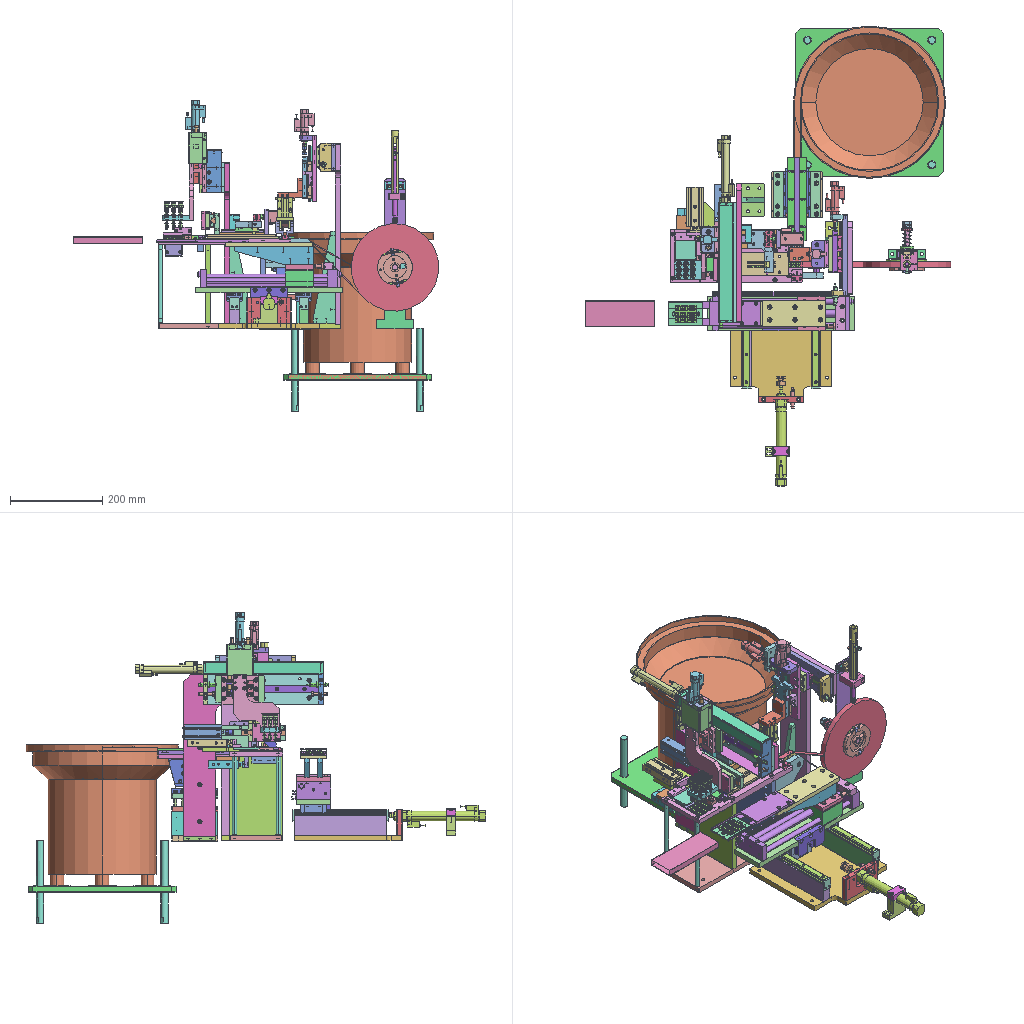Assembly | STEP file | 163 different items | 250 placed | box 792 x 996 x 674 mm
Parts list (item | name | quantity | parent item | size | volume):
1 | PN_0001 Mount electronic clip base plate | x1 | - | 115 x 233 x 12 mm | 313239 mm3
2 | PN_0002 Mount electronic clip base support plate A | x1 | - | 115 x 172 x 12 mm | 235166 mm3
3 | PN_0003 Mount electronic clip support plate B | x1 | - | 115 x 172 x 12 mm | 236361 mm3
4 | PN_0004 Mount electronic clip guide groove block | x1 | - | 287 x 115 x 14 mm | 343066 mm3
5 | PN_0005 Mount electronic clip support shaft | x2 | - | 10 x 10 x 171 mm | 13199 mm3
6 | PN_0006 Mount electronic clip pad block 3 | x1 | - | 99 x 40 x 13 mm | 46951 mm3
7 | PN_0007 Mount electronic clip cylinder mounting plate 1 | x1 | - | 40 x 62 x 8 mm | 17667 mm3
8 | PN_0008 Mount electronic clip movable head A | x1 | - | 10 x 10 x 30 mm | 1030 mm3
9 | PN_0009 Mount electronic clip movable connector head B | x1 | - | 36 x 16 x 18 mm | 5496 mm3
10 | PN_0010 Mount electronic clip quantitative slide block | x1 | - | 90 x 58 x 12 mm | 32694 mm3
11 | PN_0011 Mount electronic clip block | x1 | - | 14 x 34.832 x 10 mm | 2899 mm3
12 | PN_0012 Mount electronic clip wheel shaft A | x1 | - | 5 x 5 x 38 mm | 723.858 mm3
13 | PN_0013 Mount electronic clip mounting plate 1 | x1 | - | 160 x 54 x 10 mm | 58459 mm3
14 | PN_0014 Mount electronic clip cylinder pad block | x1 | - | 22 x 32 x 6 mm | 4030 mm3
15 | PN_0015 Mount electronic clip cylinder connecting head | x1 | - | 14 x 14 x 19 mm | 1465 mm3
16 | PN_0016 Mount electronic clip connecting block | x1 | - | 40 x 10 x 70 mm | 23648 mm3
17 | PN_0017 Mount electronic clip blade pressure plate 2 | x1 | - | 40 x 8 x 60 mm | 18433 mm3
18 | PN_0018 Mount electronic clip limit block B | x1 | - | 22 x 50 x 40 mm | 16406 mm3
19 | PN_0019 Mount electronic clip transparent acrylic cover plate | x1 | - | 152 x 50 x 8 mm | 50516 mm3
20 | PN_0021 Mount electronic clip pressure block | x2 | - | 14 x 15 x 9 mm | 1490 mm3
21 | PN_0022 Mount electronic clip pressure block | x1 | - | 22 x 8 x 31 mm | 3731 mm3
22 | PN_0023 Mount electronic clip pressure plate | x1 | - | 40 x 16 x 10 mm | 4854 mm3
23 | PN_0024 Mount electronic clip spring mounting plate | x1 | - | 54 x 12 x 15 mm | 8265 mm3
24 | PN_0025 Mount electronic clip cylinder mounting plate 4 | x1 | - | 61 x 80 x 10 mm | 39986 mm3
25 | PN_0026 Mount electronic clip cylinder connecting plate | x1 | - | 60 x 18 x 18 mm | 7277 mm3
26 | PN_0027 Mount electronic clip acrylic plate | x1 | - | 44 x 56 x 5 mm | 11600 mm3
27 | PN_0028 Mount electronic clip mounting plate 3 | x1 | - | 50 x 40 x 9 mm | 17291 mm3
28 | PN_0029 Mount electronic clip connecting plate 1 | x1 | - | 43 x 36 x 35 mm | 15801 mm3
29 | PN_0030 Mount electronic clip fiber mounting seat A | x1 | - | 22 x 18 x 8 mm | 1490 mm3
30 | PN_0031 Mount electronic clip fiber sensor seat B | x1 | - | 23 x 10 x 10 mm | 1376 mm3
31 | PN_0032 Mount electronic clip wheel connecting mounting plate | x1 | - | 98 x 64 x 12 mm | 54471 mm3
32 | PN_0033 Mount electronic clip wheel connector | x1 | - | 34 x 34 x 16.4 mm | 6483 mm3
33 | PN_0034 Mount electronic clip support wheel shaft | x1 | - | 12 x 12 x 41.3 mm | 3359 mm3
34 | PN_0038 vibratory adjusting plate A | x1 | in AAAACcBASE vibratory feeder assembly B | 100 x 100 x 10 mm | 94670 mm3
35 | PN_0037 vibratory adjusting plate B | x1 | in AAAACcBASE vibratory feeder assembly B | 100 x 10 x 100 mm | 97001 mm3
36 | A vibratory feeder 1 | x1 | in AAAA upper machine frame component | 108 x 76 x 60.4 mm | 290957 mm3
37 | ASCB6-30 | x8 | in AAAA upper machine frame component | 36 x 10 x 10 mm | 1241 mm3
38 | PN_0039 vibratory feeder connecting plate | x1 | in AAAA upper machine frame component | 140 x 8 x 40 mm | 43075 mm3
39 | PN_0036 vibratory vertical plate | x2 | in AAAA upper machine frame component | 100 x 10 x 55 mm | 54201 mm3
40 | PN_0035 vibratory base plate | x1 | in AAAA upper machine frame component | 110 x 100 x 12 mm | 122022 mm3
41 | PN_0040 linear vibrating groove | x1 | - | 180 x 40 x 10 mm | 61766 mm3
42 | PN_0041 Mount electronic clip pressure rod | x2 | - | 15 x 180 x 3 mm | 7714 mm3
43 | PN_0042 Mount electronic clip fixed groove | x1 | - | 25 x 7.5 x 40 mm | 5632 mm3
44 | PN_0043 Mount electronic clip pressure block A | x2 | - | 7.5 x 20 x 4 mm | 440.722 mm3
45 | PN_0044 Mount electronic clip mounting base plate B | x1 | - | 60 x 80 x 12 mm | 51231 mm3
46 | PN_0045 Mount electronic clip mounting plate 6 | x1 | - | 160 x 392 x 12 mm | 427849 mm3
47 | PN_0046 Mount electronic clip reinforcing rib A | x2 | - | 48 x 200 x 10 mm | 59178 mm3
48 | Mount electronic clip vibrating plate BM23-2V1 part | x1 | - | 330 x 330 x 319 mm | 10354356 mm3
49 | PN_0047 Mount electronic clip mounting base plate | x1 | in Mount electronic clip manipulator A | 60 x 10 x 175 mm | 99342 mm3
50 | MGN12C (slide rail) | x1 | in Mount electronic clip manipulator A | 12 x 8 x 145 mm | 12355 mm3
51 | Mount electronic clip MGN12C (slider) | x2 | in Mount electronic clip manipulator A | 27 x 10 x 34.7 mm | 7013 mm3
52 | PN_0048 Mount electronic clip cylinder mounting plate | x1 | in Mount electronic clip manipulator A | 60 x 28 x 10 mm | 13235 mm3
53 | PN_0049 Mount electronic clip cylinder mounting plate 2 | x1 | in Mount electronic clip manipulator A | 60 x 25 x 10 mm | 13990 mm3
54 | PN_0050 Mount electronic clip slider mounting plate | x1 | in Mount electronic clip manipulator A | 90 x 58 x 10 mm | 36578 mm3
55 | Mount electronic clip RB0806 | x2 | in Mount electronic clip manipulator A | 12 x 13.856 x 46.8 mm | 2563 mm3
56 | Mount electronic clip cylinder CDJ2B16-30-C76(0) | x1 | in Mount electronic clip manipulator A | 18.6 x 41.8 x 105 mm | 26186 mm3
57 | PN_0051 Mount electronic clip movable connector head | x2 | in Mount electronic clip manipulator A, Mount electronic clip manipulator A Z-axis | 10 x 10 x 18 mm | 883.594 mm3
58 | PN_0052 Mount electronic clip manipulator mounting plate | x1 | - | 45 x 80 x 10 mm | 30659 mm3
59 | PN_0053 Mount electronic clip mounting base plate Z-axis | x1 | in Mount electronic clip manipulator A Z-axis | 60 x 10 x 144 mm | 79878 mm3
60 | Mount electronic clip MGN12C (slide rail) Z-axis | x1 | in Mount electronic clip manipulator A Z-axis | 12 x 8 x 120 mm | 10218 mm3
61 | Mount electronic clip MGN12C (slider) Z-axis | x2 | in Mount electronic clip manipulator A Z-axis | 27 x 10 x 34.7 mm | 7013 mm3
62 | Mount electronic clip cylinder mounting plate Z-axis | x1 | in Mount electronic clip manipulator A Z-axis | 60 x 28 x 10 mm | 13269 mm3
63 | Mount electronic clip RB0806 Z-axis | x2 | in Mount electronic clip manipulator A Z-axis | 12 x 13.856 x 46.8 mm | 2563 mm3
64 | Mount electronic clip cylinder CDJ2B16-15-C76(0) Z-axis | x1 | in Mount electronic clip manipulator A Z-axis | 18.6 x 41.8 x 90 mm | 22619 mm3
65 | PN_0054 Mount electronic clip slider mounting plate Z-axis | x1 | in Mount electronic clip manipulator A Z-axis | 90 x 58 x 10 mm | 25065 mm3
66 | PN_0055 Mount electronic clip limit mounting block A | x1 | in Mount electronic clip manipulator A Z-axis | 30 x 23 x 12 mm | 3387 mm3
67 | PN_0056 Mount electronic clip limit mounting block B | x1 | in Mount electronic clip manipulator A Z-axis | 30 x 23 x 12 mm | 3584 mm3
68 | Mount electronic clip cleaning part 20141015 | x2 | - | 75 x 1.3 x 50 mm | 4576 mm3
69 | PN_0057 Mount electronic clip finger cylinder mounting plate A | x1 | - | 30 x 42 x 54 mm | 24235 mm3
70 | PN_0058 Mount electronic clip electronic clip plate | x2 | - | 16.5 x 35 x 10 mm | 2631 mm3
71 | PN_0059 Mount electronic clip mounting base plate A | x1 | - | 60 x 70 x 12 mm | 44235 mm3
72 | PN_0060 Mount electronic clip mounting plate 7 | x1 | - | 302 x 350 x 12 mm | 470281 mm3
73 | PN_0061 Mount electronic clip s horizontal manipulator base plate | x1 | in Mount electronic clip s horizontal manipulator assembly | 260 x 65 x 10 mm | 150103 mm3
74 | Mount electronic clip sEGW15SA | x2 | in Mount electronic clip s horizontal manipulator assembly | 52 x 19.5 x 45.8 mm | 24435 mm3
75 | Mount electronic clip sEGW15SA- slide rail | x1 | in Mount electronic clip s horizontal manipulator assembly | 15 x 12.5 x 240 mm | 38137 mm3
76 | PN_0062 Mount electronic clip s horizontal manipulator flange plate | x1 | in Mount electronic clip s horizontal manipulator assembly | 106 x 58 x 10 mm | 46604 mm3
77 | PN_0063 Mount electronic clip s horizontal manipulator connecting rod | x1 | in Mount electronic clip s horizontal manipulator assembly | 20 x 45 x 8 mm | 5111 mm3
78 | PN_0064 Mount electronic clip s horizontal manipulator cylinder seat | x1 | in Mount electronic clip s horizontal manipulator assembly | 10 x 90 x 32 mm | 21348 mm3
79 | PN_0065 Mount electronic clip s horizontal manipulator rear end cover | x1 | in Mount electronic clip s horizontal manipulator assembly | 10 x 90 x 32 mm | 20939 mm3
80 | PN_0066 Mount electronic clip s horizontal manipulator lower plate | x1 | in Mount electronic clip s horizontal manipulator assembly | 260 x 38 x 1.5 mm | 14742 mm3
81 | PN_0067 Mount electronic clip s horizontal manipulator upper cover | x1 | in Mount electronic clip s horizontal manipulator assembly | 33 x 260 x 26 mm | 31457 mm3
82 | Mount electronic clip sUSTH6-30 | x3 | in Mount electronic clip s horizontal manipulator assembly, Mount electronic clip s longitudinal manipulator assembly_horizontal insert | 36 x 11.5 x 10 mm | 1504 mm3
83 | Mount electronic clip sRB0806 | x2 | in Mount electronic clip s horizontal manipulator assembly | 12 x 13.856 x 46.8 mm | 2563 mm3
84 | PN_0069 Mount electronic clip s longitudinal manipulator base plate | x1 | in Mount electronic clip s longitudinal manipulator assembly_horizontal insert | 80 x 130 x 9 mm | 72069 mm3
85 | Mount electronic clip sA_CDJ2B16-30-C73(0) | x1 | in Mount electronic clip s longitudinal manipulator assembly_horizontal insert | 18.6 x 41.8 x 105 mm | 26366 mm3
86 | PN_0070 Mount electronic clip s longitudinal manipulator movable head | x1 | in Mount electronic clip s longitudinal manipulator assembly_horizontal insert | 10.8 x 13 x 14 mm | 938.634 mm3
87 | PN_0071 Mount electronic clip s longitudinal manipulator slide rail plate | x1 | in Mount electronic clip s longitudinal manipulator assembly_horizontal insert | 53 x 85 x 10 mm | 23160 mm3
88 | PN_0072 Mount electronic clip s longitudinal manipulator cylinder seat | x1 | in Mount electronic clip s longitudinal manipulator assembly_horizontal insert | 55 x 30 x 10 mm | 11604 mm3
89 | Mount electronic clip sMGN9C110 | x1 | in Mount electronic clip s longitudinal manipulator assembly_horizontal insert | 9 x 6.5 x 110 mm | 5668 mm3
90 | Mount electronic clip s MGN9C slider | x2 | in Mount electronic clip s longitudinal manipulator assembly_horizontal insert | 20 x 8 x 28.9 mm | 3355 mm3
91 | s3mm pin | x1 | in Mount electronic clip s longitudinal manipulator assembly_horizontal insert | 3 x 3 x 9 mm | 60.607 mm3
92 | Mount electronic clip sRB0806S.stp | x2 | in Mount electronic clip s longitudinal manipulator assembly_horizontal insert | 12 x 13.856 x 46.8 mm | 2563 mm3
93 | PN_0073 Mount electronic clip s longitudinal manipulator buffer seat | x1 | in Mount electronic clip s longitudinal manipulator assembly_horizontal insert | 36 x 20 x 13 mm | 3299 mm3
94 | PN_0075 Mount electronic clip s longitudinal manipulator fixture | x1 | in Mount electronic clip s longitudinal manipulator assembly_horizontal insert | 58 x 66 x 39 mm | 12822 mm3
95 | PN_0074 Mount electronic clip s longitudinal manipulator limit seat | x1 | in Mount electronic clip s longitudinal manipulator assembly_horizontal insert | 36 x 20 x 13 mm | 3451 mm3
96 | PN_0068 Mount electronic clip s horizontal manipulator movable head | x1 | in Mount electronic clip sXY assembly | 16 x 16 x 68.1 mm | 8318 mm3
97 | Mount electronic clip sCDJ2B16-100-C73 | x1 | in Mount electronic clip NG | 18.6 x 41.8 x 175 mm | 45989 mm3
98 | Mount electronic clip, black, 20141015 | x4 | - | 15 x 12 x 5.1 mm | 295.394 mm3
99 | Mount electronic clip black colour part | x33 | - | 15 x 12 x 6 mm | 501.316 mm3
100 | PN_0076 Mount electronic clip suction nozzle connecting plate | x1 | - | 126 x 100 x 10 mm | 64254 mm3
101 | PN_0077 Mount electronic clip suction nozzle mounting plate | x1 | - | 40 x 60 x 10 mm | 19887 mm3
102 | PN_0078 Mount electronic clip base plate | x1 | - | 234 x 220 x 12 mm | 553966 mm3
103 | PN_0079 transport section guide rail pad block A | x1 | - | 20 x 45 x 200 mm | 171286 mm3
104 | PN_0080 transport section guide rail pad block B | x1 | - | 20 x 46 x 200 mm | 172286 mm3
105 | PN_0081 transport cylinder mounting plate | x1 | - | 96 x 56 x 12 mm | 48456 mm3
106 | PN_0082 transport limit mounting plate | x1 | - | 60 x 56 x 10 mm | 31898 mm3
107 | PN_0083 Mount electronic clip cylinder fixed support seat A | x1 | - | 52 x 20 x 42 mm | 29893 mm3
108 | PN_0084 Mount electronic clip cylinder fixed support seat B | x1 | - | 38 x 15 x 20 mm | 7297 mm3
109 | PN_0085 Mount electronic clip slider stop plate | x4 | - | 20 x 25 x 4 mm | 1857 mm3
110 | PN_0086 transport movable connector head | x1 | - | 18 x 18 x 20 mm | 3270 mm3
111 | PN_0087 transport cylinder connecting plate | x1 | - | 80 x 44 x 12 mm | 35733 mm3
112 | PN_0088 transport section connecting plate A | x1 | - | 320 x 75 x 12 mm | 262093 mm3
113 | PN_0089 Mount electronic clip connecting plate C | x1 | - | 75 x 60 x 12 mm | 39832 mm3
114 | PN_0090 Mount electronic clip mounting plate 5 | x2 | - | 170 x 40.5 x 10 mm | 51076 mm3
115 | PN_0091 Mount electronic clip connecting plate B | x1 | - | 190 x 58 x 10 mm | 99887 mm3
116 | PN_0092 Mount electronic clip plate | x1 | - | 200 x 54 x 6 mm | 39814 mm3
117 | PN_0093 Mount electronic clip adhesive tape support plate | x1 | - | 80 x 155 x 20 mm | 141530 mm3
118 | PN_0094 limit stopper | x1 | in Mount electronic clip linear fixed assembly 20141015 | 75.261 x 75.5 x 17 mm | 37225 mm3
119 | PN_0095 limit clamp block | x2 | in Mount electronic clip linear fixed assembly 20141015 | 5.9 x 13.5 x 10.5 mm | 469.35 mm3
120 | PN_0096 fixed round plate | x1 | in Mount electronic clip linear fixed assembly 20141015 | 90 x 85 x 17 mm | 43807 mm3
121 | PN_0097 linear shaft | x1 | in Mount electronic clip linear fixed assembly 20141015 | 12 x 12 x 108 mm | 9475 mm3
122 | PN_0098 tensioning part | x1 | in Mount electronic clip linear fixed assembly 20141015 | 55 x 55 x 11.5 mm | 13631 mm3
123 | PN_0099 pin shaft | x2 | in Mount electronic clip linear fixed assembly 20141015 | 4 x 4 x 24.5 mm | 178.223 mm3
124 | Mount electronic clip MGW9H rail | x1 | - | 18 x 7 x 90 mm | 10639 mm3
125 | Mount electronic clip MGW9H slider | x1 | - | 30 x 9.1 x 50.7 mm | 9721 mm3
126 | Mount electronic clip linear-type part | x1 | - | 434.57 x 190 x 12 mm | 291791 mm3
127 | deep groove ball bearings gb_Rolling bearings 61900 GB 276-94 | x2 | - | 6 x 22 x 22 mm | 1339 mm3
128 | Mount electronic clip cylinder MHZ2-16D-Y69A (14.9) | x1 | - | 43.02 x 23.6 x 68.3 mm | 34069 mm3
129 | Mount electronic clip pin shaft | x2 | - | 3 x 3 x 17 mm | 120.166 mm3
130 | MGN12 slider | x1 | - | 27 x 10 x 34.7 mm | 7013 mm3
131 | MGN12C guide rail | x1 | - | 12 x 8 x 95 mm | 8059 mm3
132 | Mount electronic clip blade | x1 | - | 60 x 18 x 0.5 mm | 480.046 mm3
133 | Suction nozzle ZPT04UNJ6-06-A8 | x9 | - | 12 x 61 x 13.856 mm | 3226 mm3
134 | Plastic bag | x1 | - | 56 x 14 x 150 mm | 10350 mm3
135 | Mount electronic clip cylinder CXSM6-20-Z73(0) | x1 | - | 37 x 16 x 78.5 mm | 36825 mm3
136 | Mount electronic clip cylinder CXSM6-40(0) | x1 | - | 37 x 16 x 98.5 mm | 44688 mm3
137 | Mount electronic clip rodless cylinder 1-2-1 | x1 | in Mount electronic clip rodless cylinder A_CDY1S15H-200-A76H(POS._0) | 85 x 39 x 312 mm | 237778 mm3
138 | Mount electronic clip rodless cylinder 2-2-2 | x1 | in Mount electronic clip rodless cylinder A_CDY1S15H-200-A76H(POS._0) | 72 x 38 x 60 mm | 135352 mm3
139 | transport cylinder RB0806 | x3 | - | 12 x 13.856 x 46.8 mm | 2563 mm3
140 | transport section slider EGH15CA_BLOCK | x2 | in EGH15CA | 34 x 19.5 x 57.8 mm | 30496 mm3
141 | transport section slide rail EG15_RAIL | x2 | in EGH15CA | 15 x 12.5 x 200 mm | 31877 mm3
142 | Fiber sensor 1 | x2 | - | 3 x 3 x 25 mm | 113.883 mm3
143 | PN_0110 Mount electronic clip adjusting screw rod | x4 | - | 16 x 16 x 180 mm | 36003 mm3
144 | deep groove ball bearings gb_Rolling bearings 6000 GB 276-94 | x2 | - | 8 x 26 x 26 mm | 2692 mm3
145 | Spring A | x1 | - | 17.5 x 17.5 x 51.5 mm | 555.182 mm3
146 | PN_0100 Mount electronic clip blade | x1 | - | 30 x 30 x 6 mm | 3137 mm3
147 | PN_0101 Mount electronic clip clamp screw | x1 | - | 25 x 25 x 4 mm | 1589 mm3
148 | hex nuts, style 1-grades ab gb_GB_FASTENER_NUT_SNAB1 M10-N | x2 | - | 18.475 x 16 x 8.4 mm | 1367 mm3
149 | PN_0102 Mount electronic clip sensor A | x1 | in Sensor assembly | 16 x 16 x 150 mm | 14386 mm3
150 | PN_0103 Mount electronic clip sensor 1 | x1 | in Sensor assembly | 10 x 10 x 165 mm | 11828 mm3
151 | M5 screw | x1 | in Sensor assembly | 8.8 x 8.8 x 25 mm | 610.203 mm3
152 | PN_0104 Mount electronic clip sensor 2 | x1 | in Sensor assembly | 4 x 4 x 22 mm | 235.712 mm3
153 | deep groove ball bearings gb_Rolling bearings 619-5 GB 276-94 | x1 | in Sensor assembly | 4 x 13 x 13 mm | 336.475 mm3
154 | PN_0105 Mount electronic clip sensor 3 | x1 | in Sensor assembly | 6 x 6 x 10.7 mm | 215.823 mm3
155 | PN_0106 Mount electronic clip sensor 4 | x1 | in Sensor assembly | 44 x 36 x 15 mm | 19047 mm3
156 | PN_0107 Mount electronic clip sensor 5 | x1 | in Sensor assembly | 45 x 18 x 2 mm | 1418 mm3
157 | 671 | x1 | in Sensor assembly | 26.18 x 14.5 x 15.5 mm | 2180 mm3
158 | PN_0108 Mount electronic clip sensor mounting plate 1 | x1 | in Sensor assembly | 45 x 170 x 17.5 mm | 20418 mm3
159 | PN_0109 Mount electronic clip vibrating disc base plate | x1 | - | 320 x 320 x 12 mm | 1214185 mm3
160 | CDQ2B16-20D-F7NV0 | x1 | - | 43.562 x 43.562 x 54 mm | 41544 mm3
161 | CDU16-40D-A93(0) | x1 | - | 20.1 x 32 x 101 mm | 45610 mm3
162 | Assembly electronic clip CDM2BZ20-125-C76(0) | x1 | - | 24 x 47.6 x 228 mm | 84347 mm3
163 | PN_0111 buffer mounting seat | x1 | - | 75 x 15 x 20 mm | 19970 mm3
Placements (level | parent | child | x y z in mm | rotation matrix by rows):
1 | subassembly 2 | PN_0001 Mount electronic clip base plate | -262.81 -79.51 -2.283 | 0 1 0 1 0 0 0 0 -1
1 | subassembly 2 | PN_0002 Mount electronic clip base support plate A | -146.31 -79.51 82.717 | 0 0 -1 -1 0 0 0 1 0
1 | subassembly 2 | PN_0003 Mount electronic clip support plate B | -265.31 -79.51 82.717 | 0 0 -1 -1 0 0 0 1 -0
1 | subassembly 2 | PN_0004 Mount electronic clip guide groove block | -92.311 -79.51 168.717 | -1 0 0 0 -1 0 0 0 1
1 | subassembly 2 | PN_0005 Mount electronic clip support shaft | -374.31 -32.01 -2.283 | 1 0 0 0 1 0 0 0 1
1 | subassembly 2 | PN_0005 Mount electronic clip support shaft | -374.31 -127.01 -2.283 | 1 0 0 0 1 0 0 0 1
1 | subassembly 2 | PN_0006 Mount electronic clip pad block 3 | -197.81 -42.01 182.717 | 1 0 0 0 1 0 0 0 1
1 | subassembly 2 | PN_0007 Mount electronic clip cylinder mounting plate 1 | -148.31 -42.01 213.717 | 0 0 1 1 0 0 0 1 0
1 | subassembly 2 | PN_0008 Mount electronic clip movable head A | -157.31 -42.01 228.717 | 0 0 1 0.7555 0.6551 0 -0.6551 0.7555 0
1 | subassembly 2 | PN_0009 Mount electronic clip movable connector head B | -165.81 -42.01 215.717 | 0 1 0 -1 0 0 0 0 1
1 | subassembly 2 | PN_0010 Mount electronic clip quantitative slide block | -154.81 -22.01 217.717 | 0 -1 0 -1 0 0 0 0 -1
1 | subassembly 2 | PN_0011 Mount electronic clip block | -174.81 -97.01 217.717 | 0 0 1 1 0 0 0 1 0
1 | subassembly 2 | PN_0012 Mount electronic clip wheel shaft A | -169.81 -118.01 212.717 | -1 0 0 0 0 1 0 1 0
1 | subassembly 2 | PN_0013 Mount electronic clip mounting plate 1 | -247.31 -62.01 209.717 | 0 0 -1 -1 0 0 0 1 0
1 | subassembly 2 | PN_0014 Mount electronic clip cylinder pad block | -257.31 6.99 221.101 | 0 0 -1 -1 0 0 0 1 0
1 | subassembly 2 | PN_0015 Mount electronic clip cylinder connecting head | -273.31 -12.01 221.101 | -0.06304 0.998 0 0 0 -1 -0.998 -0.06304 -0
1 | subassembly 2 | PN_0016 Mount electronic clip connecting block | -272.31 -62.16 220.717 | 0 -1 0 0 0 -1 1 0 -0
1 | subassembly 2 | PN_0017 Mount electronic clip blade pressure plate 2 | -281.81 -72.16 220.717 | 0 -1 0 0 0 -1 1 0 -0
1 | subassembly 2 | PN_0018 Mount electronic clip limit block B | -214.31 -23.01 208.217 | -1 0 0 0 0 1 0 1 0
1 | subassembly 2 | PN_0019 Mount electronic clip transparent acrylic cover plate | -122.311 -97.01 182.717 | -1 0 0 0 -1 0 0 0 1
1 | subassembly 2 | PN_0021 Mount electronic clip pressure block | -285.81 -120.51 179.217 | -1 0 0 0 -1 0 0 0 1
1 | subassembly 2 | PN_0021 Mount electronic clip pressure block | -285.81 -73.51 179.217 | -1 0 0 0 -1 0 0 0 1
1 | subassembly 2 | PN_0022 Mount electronic clip pressure block | -290.81 -81.51 183.217 | 1 0 0 0 0 -1 0 1 0
1 | subassembly 2 | PN_0023 Mount electronic clip pressure plate | -314.81 -97.01 179.217 | 0 -1 0 1 0 0 0 0 1
1 | subassembly 2 | PN_0024 Mount electronic clip spring mounting plate | -287.81 -97.01 168.717 | 0 1 0 1 0 0 0 0 -1
1 | subassembly 2 | PN_0025 Mount electronic clip cylinder mounting plate 4 | -313.31 -2.01 179.217 | -1 0 0 0 -1 0 0 0 1
1 | subassembly 2 | PN_0026 Mount electronic clip cylinder connecting plate | -338.31 -27.51 197.217 | 1 0 0 0 0 -1 0 1 0
1 | subassembly 2 | PN_0027 Mount electronic clip acrylic plate | -345.81 -57.51 188.217 | -1 0 0 0 1 0 0 0 -1
1 | subassembly 2 | PN_0028 Mount electronic clip mounting plate 3 | -346.06 -17.01 159.717 | 0 1 0 -1 0 0 0 0 1
1 | subassembly 2 | PN_0029 Mount electronic clip connecting plate 1 | -346.06 -53.01 162.717 | 1 0 0 0 0 -1 0 1 0
1 | subassembly 2 | PN_0030 Mount electronic clip fiber mounting seat A | -113.811 -79.51 168.717 | 1 0 0 0 -1 0 0 0 -1
1 | subassembly 2 | PN_0031 Mount electronic clip fiber sensor seat B | -104.311 -127.01 178.717 | 1 0 0 0 1 0 0 0 1
1 | subassembly 2 | PN_0032 Mount electronic clip wheel connecting mounting plate | -97.311 -115.01 150.717 | 1 0 0 0 0 -1 0 1 -0
1 | subassembly 2 | PN_0033 Mount electronic clip wheel connector | -62.31 -90.81 164.217 | 0.2843 0.9587 0 0 0 -1 -0.9587 0.2843 -0
1 | subassembly 2 | PN_0034 Mount electronic clip support wheel shaft | -62.31 -105.21 164.217 | -0.1268 -0.9919 0 0 0 1 -0.9919 0.1268 0
1 | subassembly 2 | AAAA upper machine frame component | -172.59 220.185 -55.538 | 0 0 -1 -1 0 0 0 1 -0
2 | AAAA upper machine frame component | AAAACcBASE vibratory feeder assembly B | 167.251 294.855 -50.446 | -1 0 -0.000211 0 1 0 0.000211 0 -1
3 | AAAACcBASE vibratory feeder assembly B | PN_0038 vibratory adjusting plate A | 1.053 -161.0 17.334 | 1 0.000211 0 0 0 1 0.000211 -1 0
3 | AAAACcBASE vibratory feeder assembly B | PN_0037 vibratory adjusting plate B | 51.042 -189.0 67.344 | 1 0 -0.000211 0 1 0 0.000211 0 1
2 | AAAA upper machine frame component | A vibratory feeder 1 | 166.195 143.855 -67.78 | -1 0 0 0 1 0 0 0 -1
2 | AAAA upper machine frame component | ASCB6-30 | 191.195 145.855 -25.78 | 0 -0.3972 0.9177 -1 0 0 0 -0.9177 -0.3972
2 | AAAA upper machine frame component | ASCB6-30 | 208.195 143.855 -25.78 | 0 -0.3972 0.9177 -1 0 0 0 -0.9177 -0.3972
2 | AAAA upper machine frame component | ASCB6-30 | 208.195 143.855 -109.78 | 0 -0.3972 0.9177 -1 0 0 0 -0.9177 -0.3972
2 | AAAA upper machine frame component | ASCB6-30 | 191.195 145.855 -109.78 | 0 -0.3972 0.9177 -1 0 0 0 -0.9177 -0.3972
2 | AAAA upper machine frame component | ASCB6-30 | 141.195 145.855 -109.78 | 0 -0.3972 0.9177 -1 0 0 0 -0.9177 -0.3972
2 | AAAA upper machine frame component | ASCB6-30 | 124.195 143.855 -109.78 | 0 -0.3867 0.9222 -1 0 0 0 -0.9222 -0.3867
2 | AAAA upper machine frame component | ASCB6-30 | 124.195 143.855 -25.78 | 0 -0.3867 0.9222 -1 0 0 0 -0.9222 -0.3867
2 | AAAA upper machine frame component | ASCB6-30 | 141.195 145.855 -25.78 | 0 -0.3972 0.9177 -1 0 0 0 -0.9177 -0.3972
2 | AAAA upper machine frame component | PN_0039 vibratory feeder connecting plate | 225.695 219.855 -47.78 | 1 0 0 0 1 0 0 0 1
2 | AAAA upper machine frame component | PN_0036 vibratory vertical plate | 166.195 50.855 -97.78 | 1 0 0 0 0 1 0 -1 0
2 | AAAA upper machine frame component | PN_0036 vibratory vertical plate | 166.195 50.855 -37.78 | 1 0 0 0 0 1 0 -1 0
2 | AAAA upper machine frame component | PN_0035 vibratory base plate | 166.195 40.855 -67.78 | 0 1 0 0 0 1 1 0 0
1 | subassembly 2 | PN_0040 linear vibrating groove | -104.811 44.49 172.317 | 0 -1 0 1 0 0 0 0 1
1 | subassembly 2 | PN_0041 Mount electronic clip pressure rod | -117.311 44.49 182.317 | -1 0 0 0 -1 0 0 0 1
1 | subassembly 2 | PN_0041 Mount electronic clip pressure rod | -92.311 44.49 182.317 | -1 0 0 0 -1 0 0 0 1
1 | subassembly 2 | PN_0042 Mount electronic clip fixed groove | -104.811 -86.01 178.967 | -1 0 0 0 0 1 0 1 0
1 | subassembly 2 | PN_0043 Mount electronic clip pressure block A | -95.061 -58.01 181.717 | 1 0 0 0 1 0 0 0 1
1 | subassembly 2 | PN_0043 Mount electronic clip pressure block A | -114.561 -58.01 181.717 | -1 0 0 0 -1 0 0 0 1
1 | subassembly 2 | PN_0044 Mount electronic clip mounting base plate B | -13.81 -43.51 -14.183 | 1 0 0 0 1 0 0 0 1
1 | subassembly 2 | PN_0045 Mount electronic clip mounting plate 6 | 16.189 -83.51 191.817 | 0 0 -1 1 0 0 0 -1 -0
1 | subassembly 2 | PN_0046 Mount electronic clip reinforcing rib A | 4.189 -48.51 -2.183 | -1 0 0 0 0 1 0 1 -0
1 | subassembly 2 | Mount electronic clip vibrating plate BM23-2V1 part | 52.44 254.49 -86.183 | 1 0 0 0 1 0 0 0 1
1 | subassembly 2 | Mount electronic clip manipulator A | 1.055 -265.01 357.674 | 0 -1 0 0 0 1 -1 0 -0
2 | Mount electronic clip manipulator A | PN_0047 Mount electronic clip mounting base plate | -0.1435 1.865 100.0 | 1 0 0 0 1 0 0 0 1
2 | Mount electronic clip manipulator A | MGN12C (slide rail) | -0.1435 5.865 150.0 | 1 0 0 0 1 0 0 0 1
2 | Mount electronic clip manipulator A | Mount electronic clip MGN12C (slider) | -0.1435 5.865 212.5 | 1 0 0 0 1 0 0 0 1
2 | Mount electronic clip manipulator A | PN_0048 Mount electronic clip cylinder mounting plate | -0.1435 19.865 265.0 | 1 0 0 0 1 0 0 0 1
2 | Mount electronic clip manipulator A | PN_0049 Mount electronic clip cylinder mounting plate 2 | -0.1435 18.365 100.0 | 1 0 0 0 1 0 0 0 1
2 | Mount electronic clip manipulator A | PN_0050 Mount electronic clip slider mounting plate | -0.1435 17.865 190.0 | 0 -1 0 0 0 1 -1 0 -0
2 | Mount electronic clip manipulator A | Mount electronic clip RB0806 | 19.857 22.865 245.6 | -0.9992 0.04024 0 0.04024 0.9992 0 0 0 -1
2 | Mount electronic clip manipulator A | Mount electronic clip MGN12C (slider) | -0.1435 5.865 167.5 | 1 0 0 0 1 0 0 0 1
2 | Mount electronic clip manipulator A | Mount electronic clip cylinder CDJ2B16-30-C76(0) | -0.1435 23.865 262.0 | -1 0 0 0 1 0 0 0 -1
2 | Mount electronic clip manipulator A | PN_0051 Mount electronic clip movable connector head | -0.1435 23.865 230.0 | -0.9693 0.2459 0 -0.2459 -0.9693 0 0 0 1
2 | Mount electronic clip manipulator A | Mount electronic clip RB0806 | 15.857 22.865 120.4 | 0.9566 0.2916 0 -0.2916 0.9566 0 0 0 1
1 | subassembly 2 | PN_0052 Mount electronic clip manipulator mounting plate | -36.81 -75.01 357.817 | 0 0 1 0 1 0 -1 0 0
1 | subassembly 2 | Mount electronic clip manipulator A Z-axis | -38.945 -74.867 160.817 | 0 -1 0 1 0 0 0 0 1
2 | Mount electronic clip manipulator A Z-axis | PN_0053 Mount electronic clip mounting base plate Z-axis | -0.1435 1.865 100.0 | 1 0 0 0 1 0 0 0 1
2 | Mount electronic clip manipulator A Z-axis | Mount electronic clip MGN12C (slide rail) Z-axis | -0.1435 5.865 137.0 | 1 0 0 0 1 0 0 0 1
2 | Mount electronic clip manipulator A Z-axis | Mount electronic clip MGN12C (slider) Z-axis | -0.1435 5.865 170.5 | 1 0 0 0 1 0 0 0 1
2 | Mount electronic clip manipulator A Z-axis | Mount electronic clip cylinder mounting plate Z-axis | -0.1435 19.865 234.0 | 1 0 0 0 1 0 0 0 1
2 | Mount electronic clip manipulator A Z-axis | Mount electronic clip RB0806 Z-axis | 19.857 22.865 214.6 | -0.9783 0.2073 0 0.2073 0.9783 0 0 0 -1
2 | Mount electronic clip manipulator A Z-axis | Mount electronic clip MGN12C (slider) Z-axis | -0.1435 5.865 125.5 | 1 0 0 0 1 0 0 0 1
2 | Mount electronic clip manipulator A Z-axis | Mount electronic clip cylinder CDJ2B16-15-C76(0) Z-axis | -0.1435 23.865 231.0 | -1 0 0 0 1 0 0 0 -1
2 | Mount electronic clip manipulator A Z-axis | PN_0054 Mount electronic clip slider mounting plate Z-axis | -0.1435 17.865 148.0 | 0 1 0 0 0 1 1 0 0
2 | Mount electronic clip manipulator A Z-axis | PN_0051 Mount electronic clip movable connector head | -0.1435 23.865 203.0 | 0.9974 0.0727 0 -0.0727 0.9974 0 0 0 1
2 | Mount electronic clip manipulator A Z-axis | Mount electronic clip RB0806 Z-axis | 22.857 21.865 182.4 | -0.5974 0.802 0 -0.802 -0.5974 0 0 0 1
2 | Mount electronic clip manipulator A Z-axis | PN_0055 Mount electronic clip limit mounting block A | 16.857 17.365 152.0 | 0 0 1 0 1 0 -1 0 0
2 | Mount electronic clip manipulator A Z-axis | PN_0056 Mount electronic clip limit mounting block B | -29.143 17.365 152.0 | 0 0 1 0 1 0 -1 0 -0
1 | subassembly 2 | Mount electronic clip cleaning part 20141015 | -346.062 -204.01 174.217 | 1 0 0 0 0 -1 0 1 -0
1 | subassembly 2 | PN_0057 Mount electronic clip finger cylinder mounting plate A | -66.811 -75.01 291.317 | 0 0 -1 -1 0 0 0 1 -0
1 | subassembly 2 | PN_0058 Mount electronic clip electronic clip plate | -124.26 -70.01 193.017 | 1 0 0 0 0 -1 0 1 -0
1 | subassembly 2 | PN_0058 Mount electronic clip electronic clip plate | -85.361 -80.01 193.017 | -1 0 0 0 0 1 0 1 0
1 | subassembly 2 | PN_0059 Mount electronic clip mounting base plate A | -206.062 42.99 -14.283 | -1 0 0 0 -1 0 0 0 1
1 | subassembly 2 | PN_0060 Mount electronic clip mounting plate 7 | -236.062 -73.01 170.717 | 0 0 1 1 0 0 0 1 0
1 | subassembly 2 | Mount electronic clip NG | -24.598 -29.649 118.879 | 1 0 0 0 0 -1 0 1 0
2 | Mount electronic clip NG | Mount electronic clip sXY assembly | -287.468 296.892 115.887 | 0 0 -1 0 1 0 1 0 0
3 | Mount electronic clip sXY assembly | Mount electronic clip s horizontal manipulator assembly | -0.0 0.0 -0.0 | 1 0 0 0 1 0 0 0 1
4 | Mount electronic clip s horizontal manipulator assembly | PN_0061 Mount electronic clip s horizontal manipulator base plate | -51.526 -101.054 -76.003 | 1 0 0 0 1 0 0 0 1
4 | Mount electronic clip s horizontal manipulator assembly | Mount electronic clip sEGW15SA | -96.626 -101.054 -54.753 | 0 0 1 1 0 0 0 1 0
4 | Mount electronic clip s horizontal manipulator assembly | Mount electronic clip sEGW15SA- slide rail | -51.526 -101.054 -62.753 | 0 0 -1 -1 0 0 0 1 0
4 | Mount electronic clip s horizontal manipulator assembly | PN_0062 Mount electronic clip s horizontal manipulator flange plate | -101.525 -101.054 -47.003 | -1 0 0 0 -1 0 0 0 1
4 | Mount electronic clip s horizontal manipulator assembly | PN_0063 Mount electronic clip s horizontal manipulator connecting rod | -105.525 -69.554 -50.003 | 0 0 1 0 1 0 -1 0 -0
4 | Mount electronic clip s horizontal manipulator assembly | PN_0064 Mount electronic clip s horizontal manipulator cylinder seat | 68.475 -88.554 -53.003 | 1 0 0 0 1 0 0 0 1
4 | Mount electronic clip s horizontal manipulator assembly | PN_0065 Mount electronic clip s horizontal manipulator rear end cover | -181.525 -88.554 -53.003 | 1 0 0 0 1 0 0 0 1
4 | Mount electronic clip s horizontal manipulator assembly | Mount electronic clip sEGW15SA | -106.425 -101.054 -54.753 | 0 0 -1 -1 0 0 0 1 0
4 | Mount electronic clip s horizontal manipulator assembly | PN_0066 Mount electronic clip s horizontal manipulator lower plate | -181.525 -135.054 -76.003 | 1 0 0 0 0 -1 0 1 -0
4 | Mount electronic clip s horizontal manipulator assembly | PN_0067 Mount electronic clip s horizontal manipulator upper cover | 78.475 -68.054 -70.503 | 0 -1 0 0 0 -1 1 0 -0
4 | Mount electronic clip s horizontal manipulator assembly | Mount electronic clip sUSTH6-30 | 58.474 -111.554 -42.503 | 1 0 0 0 0.9866 -0.1633 0 0.1633 0.9866
4 | Mount electronic clip s horizontal manipulator assembly | Mount electronic clip sUSTH6-30 | -161.525 -111.554 -42.503 | -1 0 0 0 0.3818 -0.9242 0 -0.9242 -0.3818
4 | Mount electronic clip s horizontal manipulator assembly | Mount electronic clip sRB0806 | -151.525 -91.554 -42.503 | 0 0 1 0 1 0 -1 0 -0
4 | Mount electronic clip s horizontal manipulator assembly | Mount electronic clip sRB0806 | 48.474 -91.554 -42.503 | 0 0 -1 0 1 0 1 0 0
3 | Mount electronic clip sXY assembly | Mount electronic clip s longitudinal manipulator assembly_horizontal insert | -101.525 -101.054 -37.003 | 1 0 0 0 1 0 0 0 1
4 | Mount electronic clip s longitudinal manipulator assembly_horizontal insert | PN_0069 Mount electronic clip s longitudinal manipulator base plate | 0.0 -0.0 0.0 | 1 0 0 0 1 0 0 0 1
4 | Mount electronic clip s longitudinal manipulator assembly_horizontal insert | Mount electronic clip sA_CDJ2B16-30-C73(0) | 0.0 81.0 23.5 | 1 0 0 0 0 -1 0 1 -0
4 | Mount electronic clip s longitudinal manipulator assembly_horizontal insert | PN_0070 Mount electronic clip s longitudinal manipulator movable head | 0.0 65.8 23.5 | 0 1 0.004335 -1 0 0 0 -0.004335 1
4 | Mount electronic clip s longitudinal manipulator assembly_horizontal insert | PN_0071 Mount electronic clip s longitudinal manipulator slide rail plate | 0.0 28.5 17.0 | 1 0 0 0 1 0 0 0 1
4 | Mount electronic clip s longitudinal manipulator assembly_horizontal insert | PN_0072 Mount electronic clip s longitudinal manipulator cylinder seat | 0.0 86.0 22.5 | -1 0 0 0 0 1 0 1 0
4 | Mount electronic clip s longitudinal manipulator assembly_horizontal insert | Mount electronic clip sMGN9C110 | 0.0 76.0 11.25 | 1 0 0 0 0 -1 0 1 -0
4 | Mount electronic clip s longitudinal manipulator assembly_horizontal insert | Mount electronic clip s MGN9C slider | 0.0 60.45 10.0 | 1 0 0 0 0 -1 0 1 -0
4 | Mount electronic clip s longitudinal manipulator assembly_horizontal insert | Mount electronic clip s MGN9C slider | 0.0 28.45 10.0 | 1 0 0 0 0 -1 0 1 -0
4 | Mount electronic clip s longitudinal manipulator assembly_horizontal insert | s3mm pin | -7.0 -32.0 11.0 | -0.3937 -0.9193 0 -0.9193 0.3937 0 0 0 -1
4 | Mount electronic clip s longitudinal manipulator assembly_horizontal insert | Mount electronic clip sRB0806S.stp | -23.0 35.4 21.5 | 0.8875 -0.4608 0 0 0 1 -0.4608 -0.8875 -0
4 | Mount electronic clip s longitudinal manipulator assembly_horizontal insert | PN_0073 Mount electronic clip s longitudinal manipulator buffer seat | -29.5 19.0 9.0 | 0 0 -1 -1 0 0 0 1 0
4 | Mount electronic clip s longitudinal manipulator assembly_horizontal insert | Mount electronic clip sRB0806S.stp | 17.0 71.6 21.5 | 0.8268 0.5626 0 0 0 -1 -0.5626 0.8268 -0
4 | Mount electronic clip s longitudinal manipulator assembly_horizontal insert | Mount electronic clip sUSTH6-30 | -17.0 82.8 21.5 | 0 -0.9733 -0.2295 1 0 0 0 -0.2295 0.9733
4 | Mount electronic clip s longitudinal manipulator assembly_horizontal insert | PN_0075 Mount electronic clip s longitudinal manipulator fixture | -27.5 96.0 0.0 | 1 0 0 0 -1 0 0 0 -1
4 | Mount electronic clip s longitudinal manipulator assembly_horizontal insert | PN_0074 Mount electronic clip s longitudinal manipulator limit seat | 16.5 19.0 9.0 | 0 0 -1 -1 0 0 0 1 0
3 | Mount electronic clip sXY assembly | PN_0068 Mount electronic clip s horizontal manipulator movable head | -92.525 -58.054 -53.003 | 0 0 -1 -0.5325 0.8464 0 0.8464 0.5325 0
2 | Mount electronic clip NG | Mount electronic clip sCDJ2B16-100-C73 | -234.465 238.838 -57.639 | 0.6181 0.7861 0 -0.7861 0.6181 0 0 0 1
1 | subassembly 2 | Mount electronic clip, black, 20141015 | -104.811 -39.01 180.317 | -1 0 0 0 -1 0 0 0 1
1 | subassembly 2 | Mount electronic clip black colour part | -285.915 -97.01 178.666 | -0.9769 0 -0.2137 0 -1 0 -0.2137 0 0.9769
1 | subassembly 2 | PN_0076 Mount electronic clip suction nozzle connecting plate | -312.062 -79.01 296.717 | 0 0 1 0 1 0 -1 0 0
1 | subassembly 2 | PN_0077 Mount electronic clip suction nozzle mounting plate | -341.062 -109.01 221.717 | 0 1 0 -1 0 0 0 0 1
1 | subassembly 2 | PN_0078 Mount electronic clip base plate | -139.31 -279.01 -14.283 | 0 -1 0 1 0 0 0 0 1
1 | subassembly 2 | PN_0079 transport section guide rail pad block A | -214.31 -162.01 19.217 | 1 0 0 0 0 -1 0 1 -0
1 | subassembly 2 | PN_0080 transport section guide rail pad block B | -64.311 -162.01 19.717 | 1 0 0 0 0 -1 0 1 -0
1 | subassembly 2 | PN_0081 transport cylinder mounting plate | -139.31 -384.01 25.717 | 1 0 0 0 0 -1 0 1 -0
1 | subassembly 2 | PN_0082 transport limit mounting plate | -139.31 -200.01 25.717 | 1 0 0 0 0 -1 0 1 -0
1 | subassembly 2 | PN_0083 Mount electronic clip cylinder fixed support seat A | -139.31 -502.01 -2.283 | 1 0 0 0 1 0 0 0 1
1 | subassembly 2 | PN_0084 Mount electronic clip cylinder fixed support seat B | -139.31 -492.01 47.717 | 1 0 0 0 0 -1 0 1 -0
1 | subassembly 2 | PN_0085 Mount electronic clip slider stop plate | -214.31 -362.01 41.217 | 1 0 0 0 0 -1 0 1 -0
1 | subassembly 2 | PN_0086 transport movable connector head | -139.31 -339.01 39.717 | 0.6817 -0.7317 0 0 0 -1 0.7317 0.6817 -0
1 | subassembly 2 | PN_0087 transport cylinder connecting plate | -139.31 -229.01 54.217 | 1 0 0 0 0 -1 0 1 -0
1 | subassembly 2 | PN_0088 transport section connecting plate A | -139.31 -203.51 76.217 | 1 0 0 0 -1 0 0 0 -1
1 | subassembly 2 | PN_0089 Mount electronic clip connecting plate C | -73.8 -203.51 113.217 | 0 1 0 -1 0 0 0 0 1
1 | subassembly 2 | PN_0090 Mount electronic clip mounting plate 5 | -43.8 -212.51 164.717 | -1 0 0 0 0 -1 0 -1 -0
1 | subassembly 2 | PN_0090 Mount electronic clip mounting plate 5 | -43.8 -184.51 164.717 | -1 0 0 0 0 -1 0 -1 -0
1 | subassembly 2 | PN_0091 Mount electronic clip connecting plate B | -138.8 -203.51 173.717 | -1 0 0 0 1 0 0 0 -1
1 | subassembly 2 | PN_0092 Mount electronic clip plate | -283.8 -203.51 172.717 | 1 0 0 0 1 0 0 0 1
1 | subassembly 2 | PN_0093 Mount electronic clip adhesive tape support plate | 133.643 -84.01 73.217 | -1 0 0 0 0 1 0 1 0
1 | subassembly 2 | Mount electronic clip black colour part | -301.062 -97.01 177.017 | -1 0 0 0 -1 0 0 0 1
1 | subassembly 2 | Mount electronic clip linear fixed assembly 20141015 | 136.514 -4.423 119.868 | 0.1694 0.9856 0.002119 0.01251 0 -0.9999 -0.9855 0.1694 -0.01233
2 | Mount electronic clip linear fixed assembly 20141015 | PN_0094 limit stopper | -0.966 -2.94 89.582 | 0.9999 0 -0.01251 0 1 0 0.01251 0 0.9999
2 | Mount electronic clip linear fixed assembly 20141015 | PN_0095 limit clamp block | 31.906 -2.89 99.994 | 0 0.9999 -0.01251 -1 0 0 0 0.01251 0.9999
2 | Mount electronic clip linear fixed assembly 20141015 | PN_0095 limit clamp block | -36.935 -2.99 100.572 | 0 -0.5988 0.8009 1 0 0 0 0.8009 0.5988
2 | Mount electronic clip linear fixed assembly 20141015 | PN_0096 fixed round plate | -0.9284 -2.94 86.582 | 0.9999 0 -0.01251 0 1 0 0.01251 0 0.9999
2 | Mount electronic clip linear fixed assembly 20141015 | PN_0097 linear shaft | -1.179 -2.94 106.581 | 0.8338 0.5519 0.01251 0.552 -0.8338 0 0.01043 0.006905 -0.9999
2 | Mount electronic clip linear fixed assembly 20141015 | PN_0098 tensioning part | -0.9284 -2.94 86.582 | 0.9999 0 0.01251 0 -1 0 0.01251 0 -0.9999
2 | Mount electronic clip linear fixed assembly 20141015 | PN_0099 pin shaft | 31.863 -13.94 103.494 | 0.8225 -0.5688 0 0 0 1 -0.5688 -0.8225 0
2 | Mount electronic clip linear fixed assembly 20141015 | PN_0099 pin shaft | -34.132 -13.94 102.668 | 1 0 0 0 0 1 0 -1 0
1 | subassembly 2 | Mount electronic clip black colour part | -269.81 -97.01 180.517 | -1 0 0 0 -1 0 0 0 1
1 | subassembly 2 | Mount electronic clip black colour part | -254.81 -97.01 180.517 | -1 0 0 0 -1 0 0 0 1
1 | subassembly 2 | Mount electronic clip black colour part | -239.81 -97.01 180.517 | -1 0 0 0 -1 0 0 0 1
1 | subassembly 2 | Mount electronic clip black colour part | -224.81 -97.01 180.517 | -1 0 0 0 -1 0 0 0 1
1 | subassembly 2 | Mount electronic clip black colour part | -209.81 -97.01 180.517 | -1 0 0 0 -1 0 0 0 1
1 | subassembly 2 | Mount electronic clip black colour part | -194.81 -97.01 180.517 | -1 0 0 0 -1 0 0 0 1
1 | subassembly 2 | Mount electronic clip black colour part | -179.81 -97.01 180.517 | -1 0 0 0 -1 0 0 0 1
1 | subassembly 2 | Mount electronic clip black colour part | -164.81 -97.01 180.517 | -1 0 0 0 -1 0 0 0 1
1 | subassembly 2 | Mount electronic clip black colour part | -149.81 -97.01 180.517 | -1 0 0 0 -1 0 0 0 1
1 | subassembly 2 | Mount electronic clip black colour part | -134.81 -97.01 180.517 | -1 0 0 0 -1 0 0 0 1
1 | subassembly 2 | Mount electronic clip MGW9H rail | -197.31 -42.01 194.717 | 0 0 1 1 0 0 0 1 0
1 | subassembly 2 | Mount electronic clip MGW9H slider | -186.81 -42.01 194.717 | 0 0 1 1 0 0 0 1 0
1 | subassembly 2 | Mount electronic clip linear-type part | 133.643 -97.01 119.217 | 1 0 0 0 0 -1 0 1 -0
1 | subassembly 2 | deep groove ball bearings gb_Rolling bearings 61900 GB 276-94 | -62.31 -102.21 164.217 | 0 -0.8489 0.5286 1 0 0 0 0.5286 0.8489
1 | subassembly 2 | deep groove ball bearings gb_Rolling bearings 61900 GB 276-94 | -62.31 -91.81 164.217 | 0 -0.8489 0.5286 1 0 0 0 0.5286 0.8489
1 | subassembly 2 | Mount electronic clip cylinder MHZ2-16D-Y69A (14.9) | -104.811 -75.01 220.317 | -1 0 0 0 1 0 0 0 -1
1 | subassembly 2 | Mount electronic clip, black, 20141015 | -104.811 -51.01 180.317 | -1 0 0 0 -1 0 0 0 1
1 | subassembly 2 | Mount electronic clip, black, 20141015 | -104.811 -63.01 180.317 | -1 0 0 0 -1 0 0 0 1
1 | subassembly 2 | Mount electronic clip, black, 20141015 | -104.811 -75.01 180.317 | -1 0 0 0 -1 0 0 0 1
1 | subassembly 2 | Mount electronic clip pin shaft | -283.31 -107.51 183.717 | 0.9559 0.2937 0 0 0 -1 -0.2937 0.9559 0
1 | subassembly 2 | Mount electronic clip pin shaft | -283.31 -69.51 183.717 | 0.9987 0.05191 0 0 0 -1 -0.05191 0.9987 0
1 | subassembly 2 | Mount electronic clip black colour part | -316.062 -97.01 177.017 | -1 0 0 0 -1 0 0 0 1
1 | subassembly 2 | Mount electronic clip black colour part | -331.062 -97.01 177.017 | -1 0 0 0 -1 0 0 0 1
1 | subassembly 2 | Mount electronic clip black colour part | -346.062 -97.01 177.017 | -1 0 0 0 -1 0 0 0 1
1 | subassembly 2 | Mount electronic clip black colour part | -361.062 -97.01 177.017 | -1 0 0 0 -1 0 0 0 1
1 | subassembly 2 | Mount electronic clip black colour part | -331.062 -109.01 177.017 | -1 0 0 0 -1 0 0 0 1
1 | subassembly 2 | Mount electronic clip black colour part | -331.062 -121.01 177.017 | -1 0 0 0 -1 0 0 0 1
1 | subassembly 2 | Mount electronic clip black colour part | -346.062 -109.01 177.017 | -1 0 0 0 -1 0 0 0 1
1 | subassembly 2 | Mount electronic clip black colour part | -346.062 -121.01 177.017 | -1 0 0 0 -1 0 0 0 1
1 | subassembly 2 | Mount electronic clip black colour part | -361.062 -109.01 177.017 | -1 0 0 0 -1 0 0 0 1
1 | subassembly 2 | Mount electronic clip black colour part | -361.062 -121.01 177.017 | -1 0 0 0 -1 0 0 0 1
1 | subassembly 2 | MGN12 slider | -256.31 -114.66 220.717 | 0 -1 0 0 0 1 -1 0 0
1 | subassembly 2 | MGN12C guide rail | -256.31 -107.01 220.717 | 0 -1 0 0 0 -1 1 0 -0
1 | subassembly 2 | Mount electronic clip blade | -277.81 -103.654 203.794 | 0 0 1 0.7071 -0.7071 0 0.7071 0.7071 -0
1 | subassembly 2 | Mount electronic clip black colour part | -119.811 -97.01 180.517 | -1 0 0 0 -1 0 0 0 1
1 | subassembly 2 | Mount electronic clip black colour part | -104.811 -97.01 180.517 | -1 0 0 0 -1 0 0 0 1
1 | subassembly 2 | Suction nozzle ZPT04UNJ6-06-A8 | -361.062 -97.01 201.717 | 0.866 0 -0.5 -0.5 0 -0.866 0 1 -0
1 | subassembly 2 | Suction nozzle ZPT04UNJ6-06-A8 | -361.062 -109.01 201.717 | 0.866 0 -0.5 -0.5 0 -0.866 0 1 -0
1 | subassembly 2 | Suction nozzle ZPT04UNJ6-06-A8 | -361.062 -121.01 201.717 | 0.866 0 -0.5 -0.5 0 -0.866 0 1 -0
1 | subassembly 2 | Suction nozzle ZPT04UNJ6-06-A8 | -346.062 -97.01 201.717 | 0.866 0 -0.5 -0.5 0 -0.866 0 1 -0
1 | subassembly 2 | Suction nozzle ZPT04UNJ6-06-A8 | -346.062 -109.01 201.717 | 0.866 0 -0.5 -0.5 0 -0.866 0 1 -0
1 | subassembly 2 | Suction nozzle ZPT04UNJ6-06-A8 | -346.062 -121.01 201.717 | 0.866 0 -0.5 -0.5 0 -0.866 0 1 -0
1 | subassembly 2 | Suction nozzle ZPT04UNJ6-06-A8 | -331.062 -97.01 201.717 | 0.866 0 -0.5 -0.5 0 -0.866 0 1 -0
1 | subassembly 2 | Suction nozzle ZPT04UNJ6-06-A8 | -331.062 -109.01 201.717 | 0.866 0 -0.5 -0.5 0 -0.866 0 1 -0
1 | subassembly 2 | Suction nozzle ZPT04UNJ6-06-A8 | -331.062 -121.01 201.717 | 0.866 0 -0.5 -0.5 0 -0.866 0 1 -0
1 | subassembly 2 | Plastic bag | -413.562 -204.01 178.217 | 0 0 -1 -1 0 0 0 1 0
1 | subassembly 2 | Mount electronic clip black colour part | -331.062 -192.01 177.017 | -1 0 0 0 -1 0 0 0 1
1 | subassembly 2 | Mount electronic clip black colour part | -346.062 -192.01 177.017 | -1 0 0 0 -1 0 0 0 1
1 | subassembly 2 | Mount electronic clip black colour part | -361.062 -192.01 177.017 | -1 0 0 0 -1 0 0 0 1
1 | subassembly 2 | Mount electronic clip black colour part | -331.062 -204.01 177.017 | -1 0 0 0 -1 0 0 0 1
1 | subassembly 2 | Mount electronic clip black colour part | -346.062 -204.01 177.017 | -1 0 0 0 -1 0 0 0 1
1 | subassembly 2 | Mount electronic clip black colour part | -361.062 -204.01 177.017 | -1 0 0 0 -1 0 0 0 1
1 | subassembly 2 | Mount electronic clip black colour part | -331.062 -216.01 177.017 | -1 0 0 0 -1 0 0 0 1
1 | subassembly 2 | Mount electronic clip black colour part | -346.062 -216.01 177.017 | -1 0 0 0 -1 0 0 0 1
1 | subassembly 2 | Mount electronic clip black colour part | -361.062 -216.01 177.017 | -1 0 0 0 -1 0 0 0 1
1 | subassembly 2 | Mount electronic clip cylinder CXSM6-20-Z73(0) | -346.06 -40.51 159.717 | -1 0 0 0 0 -1 0 -1 0
1 | subassembly 2 | Mount electronic clip cylinder CXSM6-40(0) | -325.81 -15.01 190.217 | 1 0 0 0 0 -1 0 1 0
1 | subassembly 2 | Mount electronic clip rodless cylinder A_CDY1S15H-200-A76H(POS._0) | -28.135 -216.556 71.519 | 0 0 1 1 0 0 0 1 0
2 | Mount electronic clip rodless cylinder A_CDY1S15H-200-A76H(POS._0) | Mount electronic clip rodless cylinder 1-2-1 | 13.045 24.698 14.324 | 1 0 0 0 1 0 0 0 1
2 | Mount electronic clip rodless cylinder A_CDY1S15H-200-A76H(POS._0) | Mount electronic clip rodless cylinder 2-2-2 | 13.045 24.698 -15.666 | 1 0 0 0 1 0 0 0 1
1 | subassembly 2 | transport cylinder RB0806 | -119.311 -225.41 43.717 | -0.7261 -0.6876 0 0 0 -1 0.6876 -0.7261 -0
1 | subassembly 2 | PN_0085 Mount electronic clip slider stop plate | -214.31 -158.01 41.217 | 1 0 0 0 0 -1 0 1 -0
1 | subassembly 2 | PN_0085 Mount electronic clip slider stop plate | -64.311 -158.01 41.217 | 1 0 0 0 0 -1 0 1 -0
1 | subassembly 2 | PN_0085 Mount electronic clip slider stop plate | -64.311 -362.01 41.217 | 1 0 0 0 0 -1 0 1 -0
1 | subassembly 2 | PN_0046 Mount electronic clip reinforcing rib A | -224.062 47.99 -2.283 | 1 0 0 0 0 -1 0 1 0
1 | subassembly 2 | EGH15CA | -84.005 -216.759 52.417 | 1 0 0 0 0 -1 0 1 -0
2 | EGH15CA | transport section slider EGH15CA_BLOCK | 19.695 13.301 -33.148 | 1 0 0 0 1 0 0 0 1
2 | EGH15CA | transport section slide rail EG15_RAIL | 19.695 13.301 -4.748 | 1 0 0 0 1 0 0 0 1
1 | subassembly 2 | EGH15CA | -234.005 -216.759 52.417 | 1 0 0 0 0 -1 0 1 -0
2 | EGH15CA | transport section slider EGH15CA_BLOCK | 19.695 13.301 -33.148 | 1 0 0 0 1 0 0 0 1
2 | EGH15CA | transport section slide rail EG15_RAIL | 19.695 13.301 -4.748 | 1 0 0 0 1 0 0 0 1
1 | subassembly 2 | Mount electronic clip cleaning part 20141015 | -346.3 -203.51 174.217 | 1 0 0 0 0 -1 0 1 -0
1 | subassembly 2 | Fiber sensor 1 | -106.811 -79.51 167.317 | 1 0 0 0 1 0 0 0 1
1 | subassembly 2 | PN_0110 Mount electronic clip adjusting screw rod | 187.44 119.49 -193.183 | 0.6691 0.7432 0 -0.7432 0.6691 0 0 0 1
1 | subassembly 2 | PN_0110 Mount electronic clip adjusting screw rod | -82.561 389.49 -193.183 | 0.6691 0.7432 0 -0.7432 0.6691 0 0 0 1
1 | subassembly 2 | PN_0110 Mount electronic clip adjusting screw rod | 187.44 389.49 -193.183 | 0.6691 0.7432 0 -0.7432 0.6691 0 0 0 1
1 | subassembly 2 | PN_0110 Mount electronic clip adjusting screw rod | -82.561 119.49 -193.183 | 0.6691 0.7432 0 -0.7432 0.6691 0 0 0 1
1 | subassembly 2 | deep groove ball bearings gb_Rolling bearings 6000 GB 276-94 | 133.643 -76.01 119.217 | 0 -1 0 1 0 0 0 0 1
1 | subassembly 2 | deep groove ball bearings gb_Rolling bearings 6000 GB 276-94 | 133.643 -68.01 119.217 | 0 -1 0 1 0 0 0 0 1
1 | subassembly 2 | Spring A | 133.643 -15.664 119.217 | -0.814 -0.5809 0 0 0 -1 0.5809 -0.814 -0
1 | subassembly 2 | PN_0100 Mount electronic clip blade | 133.643 -58.01 119.217 | 0.9977 0.06823 0 0 0 -1 -0.06823 0.9977 -0
1 | subassembly 2 | PN_0101 Mount electronic clip clamp screw | 133.643 -23.81 119.217 | 0.9974 0.07257 0 0 0 1 0.07257 -0.9974 0
1 | subassembly 2 | hex nuts, style 1-grades ab gb_GB_FASTENER_NUT_SNAB1 M10-N | 133.643 -11.41 119.217 | 1 0 0 0 0 -1 0 1 -0
1 | subassembly 2 | hex nuts, style 1-grades ab gb_GB_FASTENER_NUT_SNAB1 M10-N | 133.643 -19.81 119.217 | 0.9962 0.08729 0 0 0 -1 -0.08729 0.9962 -0
1 | subassembly 2 | Sensor assembly | 136.678 -96.619 565.242 | 1 0 0 0 -1 0 0 0 -1
2 | Sensor assembly | PN_0102 Mount electronic clip sensor A | -3.036 0.3913 150.0 | 1 0 0 0 1 0 0 0 1
2 | Sensor assembly | PN_0103 Mount electronic clip sensor 1 | -3.036 0.3913 183.525 | 1 0 0 0 1 0 0 0 1
2 | Sensor assembly | M5 screw | -3.036 -4.609 198.525 | 0.866 -0.5 0 0 0 1 -0.5 -0.866 -0
2 | Sensor assembly | PN_0104 Mount electronic clip sensor 2 | -3.036 -16.609 213.525 | 1 0 0 0 0 1 0 -1 0
2 | Sensor assembly | deep groove ball bearings gb_Rolling bearings 619-5 GB 276-94 | -3.036 0.3913 344.525 | 0 0.7915 0.6112 -1 0 0 0 -0.6112 0.7915
2 | Sensor assembly | PN_0105 Mount electronic clip sensor 3 | -3.036 -4.609 344.525 | 0.4267 -0.9044 0 0 0 1 -0.9044 -0.4267 0
2 | Sensor assembly | PN_0106 Mount electronic clip sensor 4 | 0.9644 -7.609 285.0 | 0 1 0 -1 0 0 0 0 1
2 | Sensor assembly | PN_0107 Mount electronic clip sensor 5 | -3.036 -29.609 268.0 | 1 0 0 0 0 1 0 -1 -0
2 | Sensor assembly | 671 | -3.036 -27.609 269.0 | -1 0 0 0 0 1 0 1 -0
2 | Sensor assembly | PN_0108 Mount electronic clip sensor mounting plate 1 | -3.036 -29.609 339.5 | -1 0 0 0 0 -1 0 -1 0
1 | subassembly 2 | Fiber sensor 1 | -104.311 -122.01 184.717 | 0.8854 -0.4648 0 0 0 1 -0.4648 -0.8854 0
1 | subassembly 2 | PN_0109 Mount electronic clip vibrating disc base plate | 52.44 254.49 -124.183 | 1 0 0 0 1 0 0 0 1
1 | subassembly 2 | transport cylinder RB0806 | -114.311 -368.61 43.717 | 1 0 0 0 0 1 0 -1 0
1 | subassembly 2 | CDQ2B16-20D-F7NV0 | -140.31 -42.01 228.717 | 0 0 -1 0 1 0 1 0 -0
1 | subassembly 2 | CDU16-40D-A93(0) | -273.31 -4.01 221.101 | 1 0 0 0 0 -1 0 1 0
1 | subassembly 2 | Assembly electronic clip CDM2BZ20-125-C76(0) | -139.31 -377.01 39.717 | 1 0 0 0 0 1 0 -1 0
1 | subassembly 2 | transport cylinder RB0806 | -40.711 -231.01 121.717 | 0 0 -1 0.5599 0.8285 0 0.8285 -0.5599 -0
1 | subassembly 2 | PN_0111 buffer mounting seat | -20.311 -203.51 121.717 | 0 0 1 1 0 0 0 1 0